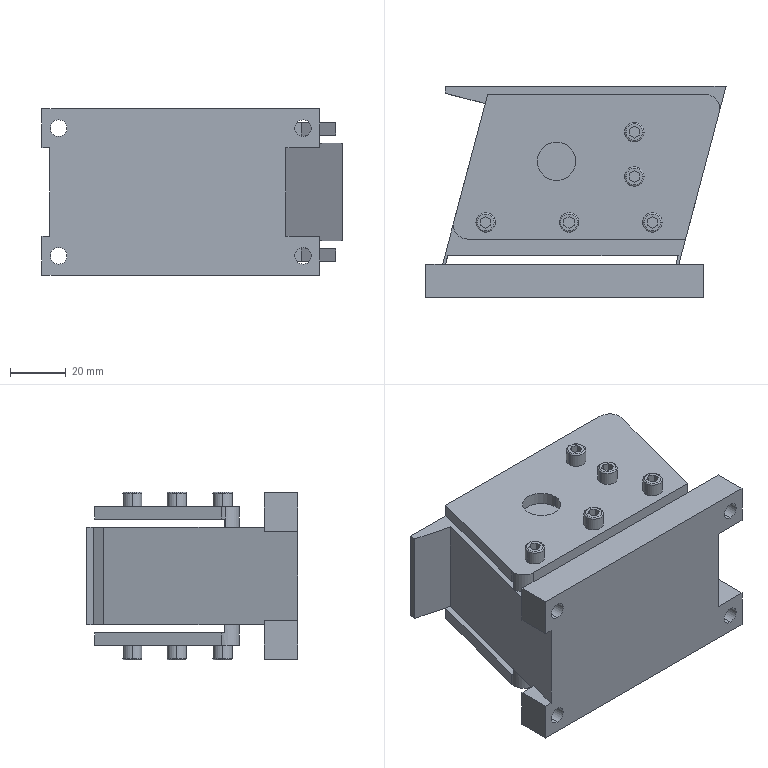Part | STEP file | A vibratory feeder 1 | 1 solid | 216 faces | box 108 x 76 x 60.4 mm | volume 290957 mm3 | plane 118 | cylinder 54 | cone 24 | torus 20 | commonest cylinder face diameters 7 x20 3.3 x8 4 x8 6 x8 10 x6 13.8 x4